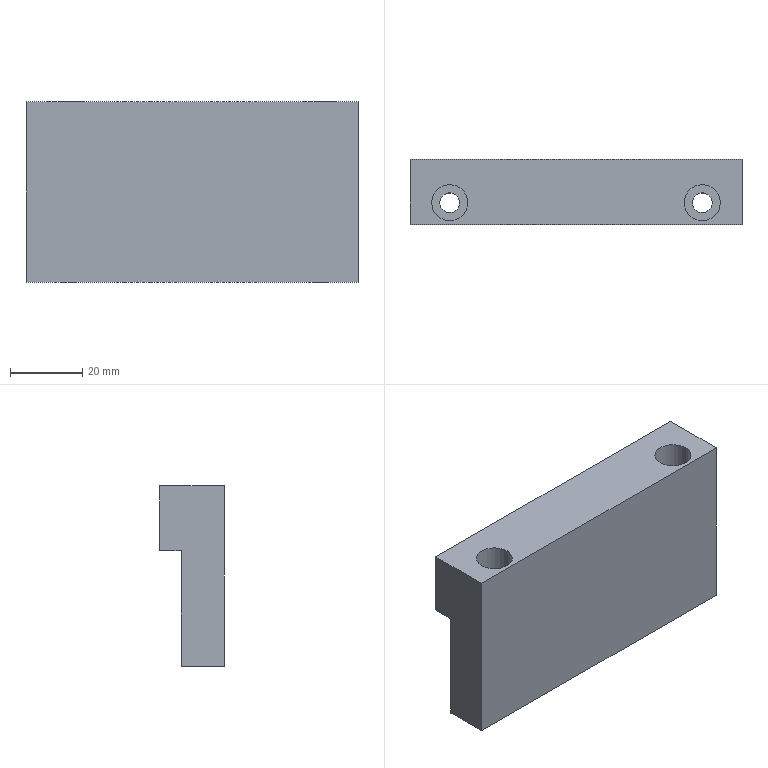Part | STEP file | 2081 Heat lower plate | 1 solid | 18 faces | box 92 x 18 x 50 mm | volume 61665 mm3 | plane 10 | cylinder 8 | commonest cylinder face diameters 5.5 x4 10 x4
STEP:
#1=CARTESIAN_POINT('',(0.,0.,0.));
#2=DIRECTION('',(0.,0.,1.));
#3=DIRECTION('',(1.,0.,0.));
#4=AXIS2_PLACEMENT_3D('',#1,#2,#3);
#5=CARTESIAN_POINT('',(-30.,-3.,8.));
#6=VERTEX_POINT('',#5);
#7=CARTESIAN_POINT('',(-30.,-3.,18.));
#8=VERTEX_POINT('',#7);
#9=CARTESIAN_POINT('',(-30.,-3.,18.));
#10=DIRECTION('',(0.,0.,1.));
#11=VECTOR('',#10,1.);
#12=LINE('',#9,#11);
#13=CARTESIAN_POINT('',(-35.,-3.,18.));
#14=DIRECTION('',(0.,0.,1.));
#15=DIRECTION('',(1.,0.,0.));
#16=AXIS2_PLACEMENT_3D('',#13,#14,#15);
#17=CYLINDRICAL_SURFACE('',#16,5.);
#18=CARTESIAN_POINT('',(6.283,0.));
#19=DIRECTION('',(0.,1.));
#20=VECTOR('',#19,1.);
#21=LINE('',#18,#20);
#22=(GEOMETRIC_REPRESENTATION_CONTEXT(2)PARAMETRIC_REPRESENTATION_CONTEXT()REPRESENTATION_CONTEXT('',''));
#23=DEFINITIONAL_REPRESENTATION('',(#21),#22);
#24=PCURVE('',#17,#23);
#25=CARTESIAN_POINT('',(-35.,-3.,18.));
#26=DIRECTION('',(0.,0.,1.));
#27=DIRECTION('',(1.,0.,0.));
#28=AXIS2_PLACEMENT_3D('',#25,#26,#27);
#29=CYLINDRICAL_SURFACE('',#28,5.);
#30=CARTESIAN_POINT('',(0.,0.));
#31=DIRECTION('',(0.,1.));
#32=VECTOR('',#31,1.);
#33=LINE('',#30,#32);
#34=(GEOMETRIC_REPRESENTATION_CONTEXT(2)PARAMETRIC_REPRESENTATION_CONTEXT()REPRESENTATION_CONTEXT('',''));
#35=DEFINITIONAL_REPRESENTATION('',(#33),#34);
#36=PCURVE('',#29,#35);
#37=SURFACE_CURVE('',#12,(#24,#36),.PCURVE_S1.);
#38=EDGE_CURVE('',#6,#8,#37,.T.);
#39=ORIENTED_EDGE('',*,*,#38,.T.);
#40=CARTESIAN_POINT('',(-40.,-3.,18.));
#41=VERTEX_POINT('',#40);
#42=CARTESIAN_POINT('',(-35.,-3.,18.));
#43=DIRECTION('',(0.,0.,1.));
#44=DIRECTION('',(1.,0.,0.));
#45=AXIS2_PLACEMENT_3D('',#42,#43,#44);
#46=CIRCLE('',#45,5.);
#47=CARTESIAN_POINT('',(0.,0.));
#48=DIRECTION('',(1.,0.));
#49=VECTOR('',#48,1.);
#50=LINE('',#47,#49);
#51=(GEOMETRIC_REPRESENTATION_CONTEXT(2)PARAMETRIC_REPRESENTATION_CONTEXT()REPRESENTATION_CONTEXT('',''));
#52=DEFINITIONAL_REPRESENTATION('',(#50),#51);
#53=PCURVE('',#17,#52);
#54=CARTESIAN_POINT('',(0.,0.,18.));
#55=DIRECTION('',(0.,0.,-1.));
#56=DIRECTION('',(-1.,0.,0.));
#57=AXIS2_PLACEMENT_3D('',#54,#55,#56);
#58=PLANE('',#57);
#59=CARTESIAN_POINT('',(30.,-3.));
#60=CARTESIAN_POINT('',(30.,5.66));
#61=CARTESIAN_POINT('',(37.5,1.33));
#62=CARTESIAN_POINT('',(45.,-3.));
#63=CARTESIAN_POINT('',(37.5,-7.33));
#64=CARTESIAN_POINT('',(30.,-11.66));
#65=CARTESIAN_POINT('',(30.,-3.));
#66=(BOUNDED_CURVE()B_SPLINE_CURVE(2,(#59,#60,#61,#62,#63,#64,#65),.UNSPECIFIED.,.T.,.F.)B_SPLINE_CURVE_WITH_KNOTS((1,2,2,2,2,1),(-2.094,0.,2.094,4.189,6.283,8.378),.UNSPECIFIED.)CURVE()GEOMETRIC_REPRESENTATION_ITEM()RATIONAL_B_SPLINE_CURVE((1.,0.5,1.,0.5,1.,0.5,1.))REPRESENTATION_ITEM(''));
#67=(GEOMETRIC_REPRESENTATION_CONTEXT(2)PARAMETRIC_REPRESENTATION_CONTEXT()REPRESENTATION_CONTEXT('',''));
#68=DEFINITIONAL_REPRESENTATION('',(#66),#67);
#69=PCURVE('',#58,#68);
#70=SURFACE_CURVE('',#46,(#53,#69),.PCURVE_S1.);
#71=EDGE_CURVE('',#41,#8,#70,.T.);
#72=ORIENTED_EDGE('',*,*,#71,.F.);
#73=CARTESIAN_POINT('',(-40.,-3.,8.));
#74=VERTEX_POINT('',#73);
#75=CARTESIAN_POINT('',(-40.,-3.,18.));
#76=DIRECTION('',(0.,0.,1.));
#77=VECTOR('',#76,1.);
#78=LINE('',#75,#77);
#79=CARTESIAN_POINT('',(3.142,0.));
#80=DIRECTION('',(0.,1.));
#81=VECTOR('',#80,1.);
#82=LINE('',#79,#81);
#83=(GEOMETRIC_REPRESENTATION_CONTEXT(2)PARAMETRIC_REPRESENTATION_CONTEXT()REPRESENTATION_CONTEXT('',''));
#84=DEFINITIONAL_REPRESENTATION('',(#82),#83);
#85=PCURVE('',#17,#84);
#86=CARTESIAN_POINT('',(3.142,0.));
#87=DIRECTION('',(0.,1.));
#88=VECTOR('',#87,1.);
#89=LINE('',#86,#88);
#90=(GEOMETRIC_REPRESENTATION_CONTEXT(2)PARAMETRIC_REPRESENTATION_CONTEXT()REPRESENTATION_CONTEXT('',''));
#91=DEFINITIONAL_REPRESENTATION('',(#89),#90);
#92=PCURVE('',#29,#91);
#93=SURFACE_CURVE('',#78,(#85,#92),.PCURVE_S1.);
#94=EDGE_CURVE('',#74,#41,#93,.T.);
#95=ORIENTED_EDGE('',*,*,#94,.F.);
#96=CARTESIAN_POINT('',(-35.,-3.,8.));
#97=DIRECTION('',(0.,0.,1.));
#98=DIRECTION('',(1.,0.,0.));
#99=AXIS2_PLACEMENT_3D('',#96,#97,#98);
#100=CIRCLE('',#99,5.);
#101=CARTESIAN_POINT('',(0.,-10.));
#102=DIRECTION('',(1.,0.));
#103=VECTOR('',#102,1.);
#104=LINE('',#101,#103);
#105=(GEOMETRIC_REPRESENTATION_CONTEXT(2)PARAMETRIC_REPRESENTATION_CONTEXT()REPRESENTATION_CONTEXT('',''));
#106=DEFINITIONAL_REPRESENTATION('',(#104),#105);
#107=PCURVE('',#17,#106);
#108=CARTESIAN_POINT('',(-32.25,-3.,8.));
#109=DIRECTION('',(0.,0.,-1.));
#110=DIRECTION('',(-1.,0.,0.));
#111=AXIS2_PLACEMENT_3D('',#108,#109,#110);
#112=PLANE('',#111);
#113=CARTESIAN_POINT('',(-2.25,0.));
#114=CARTESIAN_POINT('',(-2.25,8.66));
#115=CARTESIAN_POINT('',(5.25,4.33));
#116=CARTESIAN_POINT('',(12.75,0.));
#117=CARTESIAN_POINT('',(5.25,-4.33));
#118=CARTESIAN_POINT('',(-2.25,-8.66));
#119=CARTESIAN_POINT('',(-2.25,0.));
#120=(BOUNDED_CURVE()B_SPLINE_CURVE(2,(#113,#114,#115,#116,#117,#118,#119),.UNSPECIFIED.,.T.,.F.)B_SPLINE_CURVE_WITH_KNOTS((1,2,2,2,2,1),(-2.094,0.,2.094,4.189,6.283,8.378),.UNSPECIFIED.)CURVE()GEOMETRIC_REPRESENTATION_ITEM()RATIONAL_B_SPLINE_CURVE((1.,0.5,1.,0.5,1.,0.5,1.))REPRESENTATION_ITEM(''));
#121=(GEOMETRIC_REPRESENTATION_CONTEXT(2)PARAMETRIC_REPRESENTATION_CONTEXT()REPRESENTATION_CONTEXT('',''));
#122=DEFINITIONAL_REPRESENTATION('',(#120),#121);
#123=PCURVE('',#112,#122);
#124=SURFACE_CURVE('',#100,(#107,#123),.PCURVE_S1.);
#125=EDGE_CURVE('',#74,#6,#124,.T.);
#126=ORIENTED_EDGE('',*,*,#125,.T.);
#127=EDGE_LOOP('',(#39,#72,#95,#126));
#128=FACE_BOUND('',#127,.F.);
#129=ADVANCED_FACE('',(#128),#17,.F.);
#130=CARTESIAN_POINT('',(-32.25,-3.,-32.));
#131=VERTEX_POINT('',#130);
#132=CARTESIAN_POINT('',(-32.25,-3.,8.));
#133=VERTEX_POINT('',#132);
#134=CARTESIAN_POINT('',(-32.25,-3.,18.));
#135=DIRECTION('',(0.,0.,1.));
#136=VECTOR('',#135,1.);
#137=LINE('',#134,#136);
#138=CARTESIAN_POINT('',(-35.,-3.,18.));
#139=DIRECTION('',(0.,0.,1.));
#140=DIRECTION('',(1.,0.,0.));
#141=AXIS2_PLACEMENT_3D('',#138,#139,#140);
#142=CYLINDRICAL_SURFACE('',#141,2.75);
#143=CARTESIAN_POINT('',(6.283,0.));
#144=DIRECTION('',(0.,1.));
#145=VECTOR('',#144,1.);
#146=LINE('',#143,#145);
#147=(GEOMETRIC_REPRESENTATION_CONTEXT(2)PARAMETRIC_REPRESENTATION_CONTEXT()REPRESENTATION_CONTEXT('',''));
#148=DEFINITIONAL_REPRESENTATION('',(#146),#147);
#149=PCURVE('',#142,#148);
#150=CARTESIAN_POINT('',(-35.,-3.,18.));
#151=DIRECTION('',(0.,0.,1.));
#152=DIRECTION('',(1.,0.,0.));
#153=AXIS2_PLACEMENT_3D('',#150,#151,#152);
#154=CYLINDRICAL_SURFACE('',#153,2.75);
#155=CARTESIAN_POINT('',(0.,0.));
#156=DIRECTION('',(0.,1.));
#157=VECTOR('',#156,1.);
#158=LINE('',#155,#157);
#159=(GEOMETRIC_REPRESENTATION_CONTEXT(2)PARAMETRIC_REPRESENTATION_CONTEXT()REPRESENTATION_CONTEXT('',''));
#160=DEFINITIONAL_REPRESENTATION('',(#158),#159);
#161=PCURVE('',#154,#160);
#162=SURFACE_CURVE('',#137,(#149,#161),.PCURVE_S1.);
#163=EDGE_CURVE('',#131,#133,#162,.T.);
#164=ORIENTED_EDGE('',*,*,#163,.T.);
#165=CARTESIAN_POINT('',(-37.75,-3.,8.));
#166=VERTEX_POINT('',#165);
#167=CARTESIAN_POINT('',(-35.,-3.,8.));
#168=DIRECTION('',(0.,0.,1.));
#169=DIRECTION('',(1.,0.,0.));
#170=AXIS2_PLACEMENT_3D('',#167,#168,#169);
#171=CIRCLE('',#170,2.75);
#172=CARTESIAN_POINT('',(0.,-10.));
#173=DIRECTION('',(1.,0.));
#174=VECTOR('',#173,1.);
#175=LINE('',#172,#174);
#176=(GEOMETRIC_REPRESENTATION_CONTEXT(2)PARAMETRIC_REPRESENTATION_CONTEXT()REPRESENTATION_CONTEXT('',''));
#177=DEFINITIONAL_REPRESENTATION('',(#175),#176);
#178=PCURVE('',#142,#177);
#179=CARTESIAN_POINT('',(0.,0.));
#180=CARTESIAN_POINT('',(0.,4.763));
#181=CARTESIAN_POINT('',(4.125,2.382));
#182=CARTESIAN_POINT('',(8.25,0.));
#183=CARTESIAN_POINT('',(4.125,-2.382));
#184=CARTESIAN_POINT('',(0.,-4.763));
#185=CARTESIAN_POINT('',(0.,0.));
#186=(BOUNDED_CURVE()B_SPLINE_CURVE(2,(#179,#180,#181,#182,#183,#184,#185),.UNSPECIFIED.,.T.,.F.)B_SPLINE_CURVE_WITH_KNOTS((1,2,2,2,2,1),(-2.094,0.,2.094,4.189,6.283,8.378),.UNSPECIFIED.)CURVE()GEOMETRIC_REPRESENTATION_ITEM()RATIONAL_B_SPLINE_CURVE((1.,0.5,1.,0.5,1.,0.5,1.))REPRESENTATION_ITEM(''));
#187=(GEOMETRIC_REPRESENTATION_CONTEXT(2)PARAMETRIC_REPRESENTATION_CONTEXT()REPRESENTATION_CONTEXT('',''));
#188=DEFINITIONAL_REPRESENTATION('',(#186),#187);
#189=PCURVE('',#112,#188);
#190=SURFACE_CURVE('',#171,(#178,#189),.PCURVE_S1.);
#191=EDGE_CURVE('',#166,#133,#190,.T.);
#192=ORIENTED_EDGE('',*,*,#191,.F.);
#193=CARTESIAN_POINT('',(-37.75,-3.,-32.));
#194=VERTEX_POINT('',#193);
#195=CARTESIAN_POINT('',(-37.75,-3.,18.));
#196=DIRECTION('',(0.,0.,1.));
#197=VECTOR('',#196,1.);
#198=LINE('',#195,#197);
#199=CARTESIAN_POINT('',(3.142,0.));
#200=DIRECTION('',(0.,1.));
#201=VECTOR('',#200,1.);
#202=LINE('',#199,#201);
#203=(GEOMETRIC_REPRESENTATION_CONTEXT(2)PARAMETRIC_REPRESENTATION_CONTEXT()REPRESENTATION_CONTEXT('',''));
#204=DEFINITIONAL_REPRESENTATION('',(#202),#203);
#205=PCURVE('',#142,#204);
#206=CARTESIAN_POINT('',(3.142,0.));
#207=DIRECTION('',(0.,1.));
#208=VECTOR('',#207,1.);
#209=LINE('',#206,#208);
#210=(GEOMETRIC_REPRESENTATION_CONTEXT(2)PARAMETRIC_REPRESENTATION_CONTEXT()REPRESENTATION_CONTEXT('',''));
#211=DEFINITIONAL_REPRESENTATION('',(#209),#210);
#212=PCURVE('',#154,#211);
#213=SURFACE_CURVE('',#198,(#205,#212),.PCURVE_S1.);
#214=EDGE_CURVE('',#194,#166,#213,.T.);
#215=ORIENTED_EDGE('',*,*,#214,.F.);
#216=CARTESIAN_POINT('',(-35.,-3.,-32.));
#217=DIRECTION('',(0.,0.,1.));
#218=DIRECTION('',(1.,0.,0.));
#219=AXIS2_PLACEMENT_3D('',#216,#217,#218);
#220=CIRCLE('',#219,2.75);
#221=CARTESIAN_POINT('',(0.,-50.));
#222=DIRECTION('',(1.,0.));
#223=VECTOR('',#222,1.);
#224=LINE('',#221,#223);
#225=(GEOMETRIC_REPRESENTATION_CONTEXT(2)PARAMETRIC_REPRESENTATION_CONTEXT()REPRESENTATION_CONTEXT('',''));
#226=DEFINITIONAL_REPRESENTATION('',(#224),#225);
#227=PCURVE('',#142,#226);
#228=CARTESIAN_POINT('',(0.,0.,-32.));
#229=DIRECTION('',(0.,0.,1.));
#230=DIRECTION('',(1.,0.,0.));
#231=AXIS2_PLACEMENT_3D('',#228,#229,#230);
#232=PLANE('',#231);
#233=CARTESIAN_POINT('',(-35.,-3.));
#234=DIRECTION('',(1.,0.));
#235=AXIS2_PLACEMENT_2D('',#233,#234);
#236=CIRCLE('',#235,2.75);
#237=(GEOMETRIC_REPRESENTATION_CONTEXT(2)PARAMETRIC_REPRESENTATION_CONTEXT()REPRESENTATION_CONTEXT('',''));
#238=DEFINITIONAL_REPRESENTATION('',(#236),#237);
#239=PCURVE('',#232,#238);
#240=SURFACE_CURVE('',#220,(#227,#239),.PCURVE_S1.);
#241=EDGE_CURVE('',#194,#131,#240,.T.);
#242=ORIENTED_EDGE('',*,*,#241,.T.);
#243=EDGE_LOOP('',(#164,#192,#215,#242));
#244=FACE_BOUND('',#243,.F.);
#245=ADVANCED_FACE('',(#244),#142,.F.);
#246=CARTESIAN_POINT('',(40.,-3.,8.));
#247=VERTEX_POINT('',#246);
#248=CARTESIAN_POINT('',(40.,-3.,18.));
#249=VERTEX_POINT('',#248);
#250=CARTESIAN_POINT('',(40.,-3.,18.));
#251=DIRECTION('',(0.,0.,1.));
#252=VECTOR('',#251,1.);
#253=LINE('',#250,#252);
#254=CARTESIAN_POINT('',(35.,-3.,18.));
#255=DIRECTION('',(0.,0.,1.));
#256=DIRECTION('',(1.,0.,0.));
#257=AXIS2_PLACEMENT_3D('',#254,#255,#256);
#258=CYLINDRICAL_SURFACE('',#257,5.);
#259=CARTESIAN_POINT('',(6.283,0.));
#260=DIRECTION('',(0.,1.));
#261=VECTOR('',#260,1.);
#262=LINE('',#259,#261);
#263=(GEOMETRIC_REPRESENTATION_CONTEXT(2)PARAMETRIC_REPRESENTATION_CONTEXT()REPRESENTATION_CONTEXT('',''));
#264=DEFINITIONAL_REPRESENTATION('',(#262),#263);
#265=PCURVE('',#258,#264);
#266=CARTESIAN_POINT('',(35.,-3.,18.));
#267=DIRECTION('',(0.,0.,1.));
#268=DIRECTION('',(1.,0.,0.));
#269=AXIS2_PLACEMENT_3D('',#266,#267,#268);
#270=CYLINDRICAL_SURFACE('',#269,5.);
#271=CARTESIAN_POINT('',(0.,0.));
#272=DIRECTION('',(0.,1.));
#273=VECTOR('',#272,1.);
#274=LINE('',#271,#273);
#275=(GEOMETRIC_REPRESENTATION_CONTEXT(2)PARAMETRIC_REPRESENTATION_CONTEXT()REPRESENTATION_CONTEXT('',''));
#276=DEFINITIONAL_REPRESENTATION('',(#274),#275);
#277=PCURVE('',#270,#276);
#278=SURFACE_CURVE('',#253,(#265,#277),.PCURVE_S1.);
#279=EDGE_CURVE('',#247,#249,#278,.T.);
#280=ORIENTED_EDGE('',*,*,#279,.T.);
#281=CARTESIAN_POINT('',(30.,-3.,18.));
#282=VERTEX_POINT('',#281);
#283=CARTESIAN_POINT('',(35.,-3.,18.));
#284=DIRECTION('',(0.,0.,1.));
#285=DIRECTION('',(1.,0.,0.));
#286=AXIS2_PLACEMENT_3D('',#283,#284,#285);
#287=CIRCLE('',#286,5.);
#288=CARTESIAN_POINT('',(0.,0.));
#289=DIRECTION('',(1.,0.));
#290=VECTOR('',#289,1.);
#291=LINE('',#288,#290);
#292=(GEOMETRIC_REPRESENTATION_CONTEXT(2)PARAMETRIC_REPRESENTATION_CONTEXT()REPRESENTATION_CONTEXT('',''));
#293=DEFINITIONAL_REPRESENTATION('',(#291),#292);
#294=PCURVE('',#258,#293);
#295=CARTESIAN_POINT('',(-40.,-3.));
#296=CARTESIAN_POINT('',(-40.,5.66));
#297=CARTESIAN_POINT('',(-32.5,1.33));
#298=CARTESIAN_POINT('',(-25.,-3.));
#299=CARTESIAN_POINT('',(-32.5,-7.33));
#300=CARTESIAN_POINT('',(-40.,-11.66));
#301=CARTESIAN_POINT('',(-40.,-3.));
#302=(BOUNDED_CURVE()B_SPLINE_CURVE(2,(#295,#296,#297,#298,#299,#300,#301),.UNSPECIFIED.,.T.,.F.)B_SPLINE_CURVE_WITH_KNOTS((1,2,2,2,2,1),(-2.094,0.,2.094,4.189,6.283,8.378),.UNSPECIFIED.)CURVE()GEOMETRIC_REPRESENTATION_ITEM()RATIONAL_B_SPLINE_CURVE((1.,0.5,1.,0.5,1.,0.5,1.))REPRESENTATION_ITEM(''));
#303=(GEOMETRIC_REPRESENTATION_CONTEXT(2)PARAMETRIC_REPRESENTATION_CONTEXT()REPRESENTATION_CONTEXT('',''));
#304=DEFINITIONAL_REPRESENTATION('',(#302),#303);
#305=PCURVE('',#58,#304);
#306=SURFACE_CURVE('',#287,(#294,#305),.PCURVE_S1.);
#307=EDGE_CURVE('',#282,#249,#306,.T.);
#308=ORIENTED_EDGE('',*,*,#307,.F.);
#309=CARTESIAN_POINT('',(30.,-3.,8.));
#310=VERTEX_POINT('',#309);
#311=CARTESIAN_POINT('',(30.,-3.,18.));
#312=DIRECTION('',(0.,0.,1.));
#313=VECTOR('',#312,1.);
#314=LINE('',#311,#313);
#315=CARTESIAN_POINT('',(3.142,0.));
#316=DIRECTION('',(0.,1.));
#317=VECTOR('',#316,1.);
#318=LINE('',#315,#317);
#319=(GEOMETRIC_REPRESENTATION_CONTEXT(2)PARAMETRIC_REPRESENTATION_CONTEXT()REPRESENTATION_CONTEXT('',''));
#320=DEFINITIONAL_REPRESENTATION('',(#318),#319);
#321=PCURVE('',#258,#320);
#322=CARTESIAN_POINT('',(3.142,0.));
#323=DIRECTION('',(0.,1.));
#324=VECTOR('',#323,1.);
#325=LINE('',#322,#324);
#326=(GEOMETRIC_REPRESENTATION_CONTEXT(2)PARAMETRIC_REPRESENTATION_CONTEXT()REPRESENTATION_CONTEXT('',''));
#327=DEFINITIONAL_REPRESENTATION('',(#325),#326);
#328=PCURVE('',#270,#327);
#329=SURFACE_CURVE('',#314,(#321,#328),.PCURVE_S1.);
#330=EDGE_CURVE('',#310,#282,#329,.T.);
#331=ORIENTED_EDGE('',*,*,#330,.F.);
#332=CARTESIAN_POINT('',(35.,-3.,8.));
#333=DIRECTION('',(0.,0.,1.));
#334=DIRECTION('',(1.,0.,0.));
#335=AXIS2_PLACEMENT_3D('',#332,#333,#334);
#336=CIRCLE('',#335,5.);
#337=CARTESIAN_POINT('',(0.,-10.));
#338=DIRECTION('',(1.,0.));
#339=VECTOR('',#338,1.);
#340=LINE('',#337,#339);
#341=(GEOMETRIC_REPRESENTATION_CONTEXT(2)PARAMETRIC_REPRESENTATION_CONTEXT()REPRESENTATION_CONTEXT('',''));
#342=DEFINITIONAL_REPRESENTATION('',(#340),#341);
#343=PCURVE('',#258,#342);
#344=CARTESIAN_POINT('',(37.75,-3.,8.));
#345=DIRECTION('',(0.,0.,-1.));
#346=DIRECTION('',(-1.,0.,0.));
#347=AXIS2_PLACEMENT_3D('',#344,#345,#346);
#348=PLANE('',#347);
#349=CARTESIAN_POINT('',(-2.25,0.));
#350=CARTESIAN_POINT('',(-2.25,8.66));
#351=CARTESIAN_POINT('',(5.25,4.33));
#352=CARTESIAN_POINT('',(12.75,0.));
#353=CARTESIAN_POINT('',(5.25,-4.33));
#354=CARTESIAN_POINT('',(-2.25,-8.66));
#355=CARTESIAN_POINT('',(-2.25,0.));
#356=(BOUNDED_CURVE()B_SPLINE_CURVE(2,(#349,#350,#351,#352,#353,#354,#355),.UNSPECIFIED.,.T.,.F.)B_SPLINE_CURVE_WITH_KNOTS((1,2,2,2,2,1),(-2.094,0.,2.094,4.189,6.283,8.378),.UNSPECIFIED.)CURVE()GEOMETRIC_REPRESENTATION_ITEM()RATIONAL_B_SPLINE_CURVE((1.,0.5,1.,0.5,1.,0.5,1.))REPRESENTATION_ITEM(''));
#357=(GEOMETRIC_REPRESENTATION_CONTEXT(2)PARAMETRIC_REPRESENTATION_CONTEXT()REPRESENTATION_CONTEXT('',''));
#358=DEFINITIONAL_REPRESENTATION('',(#356),#357);
#359=PCURVE('',#348,#358);
#360=SURFACE_CURVE('',#336,(#343,#359),.PCURVE_S1.);
#361=EDGE_CURVE('',#310,#247,#360,.T.);
#362=ORIENTED_EDGE('',*,*,#361,.T.);
#363=EDGE_LOOP('',(#280,#308,#331,#362));
#364=FACE_BOUND('',#363,.F.);
#365=ADVANCED_FACE('',(#364),#258,.F.);
#366=CARTESIAN_POINT('',(37.75,-3.,-32.));
#367=VERTEX_POINT('',#366);
#368=CARTESIAN_POINT('',(37.75,-3.,8.));
#369=VERTEX_POINT('',#368);
#370=CARTESIAN_POINT('',(37.75,-3.,18.));
#371=DIRECTION('',(0.,0.,1.));
#372=VECTOR('',#371,1.);
#373=LINE('',#370,#372);
#374=CARTESIAN_POINT('',(35.,-3.,18.));
#375=DIRECTION('',(0.,0.,1.));
#376=DIRECTION('',(1.,0.,0.));
#377=AXIS2_PLACEMENT_3D('',#374,#375,#376);
#378=CYLINDRICAL_SURFACE('',#377,2.75);
#379=CARTESIAN_POINT('',(6.283,0.));
#380=DIRECTION('',(0.,1.));
#381=VECTOR('',#380,1.);
#382=LINE('',#379,#381);
#383=(GEOMETRIC_REPRESENTATION_CONTEXT(2)PARAMETRIC_REPRESENTATION_CONTEXT()REPRESENTATION_CONTEXT('',''));
#384=DEFINITIONAL_REPRESENTATION('',(#382),#383);
#385=PCURVE('',#378,#384);
#386=CARTESIAN_POINT('',(35.,-3.,18.));
#387=DIRECTION('',(0.,0.,1.));
#388=DIRECTION('',(1.,0.,0.));
#389=AXIS2_PLACEMENT_3D('',#386,#387,#388);
#390=CYLINDRICAL_SURFACE('',#389,2.75);
#391=CARTESIAN_POINT('',(0.,0.));
#392=DIRECTION('',(0.,1.));
#393=VECTOR('',#392,1.);
#394=LINE('',#391,#393);
#395=(GEOMETRIC_REPRESENTATION_CONTEXT(2)PARAMETRIC_REPRESENTATION_CONTEXT()REPRESENTATION_CONTEXT('',''));
#396=DEFINITIONAL_REPRESENTATION('',(#394),#395);
#397=PCURVE('',#390,#396);
#398=SURFACE_CURVE('',#373,(#385,#397),.PCURVE_S1.);
#399=EDGE_CURVE('',#367,#369,#398,.T.);
#400=ORIENTED_EDGE('',*,*,#399,.T.);
#401=CARTESIAN_POINT('',(32.25,-3.,8.));
#402=VERTEX_POINT('',#401);
#403=CARTESIAN_POINT('',(35.,-3.,8.));
#404=DIRECTION('',(0.,0.,1.));
#405=DIRECTION('',(1.,0.,0.));
#406=AXIS2_PLACEMENT_3D('',#403,#404,#405);
#407=CIRCLE('',#406,2.75);
#408=CARTESIAN_POINT('',(0.,-10.));
#409=DIRECTION('',(1.,0.));
#410=VECTOR('',#409,1.);
#411=LINE('',#408,#410);
#412=(GEOMETRIC_REPRESENTATION_CONTEXT(2)PARAMETRIC_REPRESENTATION_CONTEXT()REPRESENTATION_CONTEXT('',''));
#413=DEFINITIONAL_REPRESENTATION('',(#411),#412);
#414=PCURVE('',#378,#413);
#415=CARTESIAN_POINT('',(0.,0.));
#416=CARTESIAN_POINT('',(0.,4.763));
#417=CARTESIAN_POINT('',(4.125,2.382));
#418=CARTESIAN_POINT('',(8.25,0.));
#419=CARTESIAN_POINT('',(4.125,-2.382));
#420=CARTESIAN_POINT('',(0.,-4.763));
#421=CARTESIAN_POINT('',(0.,0.));
#422=(BOUNDED_CURVE()B_SPLINE_CURVE(2,(#415,#416,#417,#418,#419,#420,#421),.UNSPECIFIED.,.T.,.F.)B_SPLINE_CURVE_WITH_KNOTS((1,2,2,2,2,1),(-2.094,0.,2.094,4.189,6.283,8.378),.UNSPECIFIED.)CURVE()GEOMETRIC_REPRESENTATION_ITEM()RATIONAL_B_SPLINE_CURVE((1.,0.5,1.,0.5,1.,0.5,1.))REPRESENTATION_ITEM(''));
#423=(GEOMETRIC_REPRESENTATION_CONTEXT(2)PARAMETRIC_REPRESENTATION_CONTEXT()REPRESENTATION_CONTEXT('',''));
#424=DEFINITIONAL_REPRESENTATION('',(#422),#423);
#425=PCURVE('',#348,#424);
#426=SURFACE_CURVE('',#407,(#414,#425),.PCURVE_S1.);
#427=EDGE_CURVE('',#402,#369,#426,.T.);
#428=ORIENTED_EDGE('',*,*,#427,.F.);
#429=CARTESIAN_POINT('',(32.25,-3.,-32.));
#430=VERTEX_POINT('',#429);
#431=CARTESIAN_POINT('',(32.25,-3.,18.));
#432=DIRECTION('',(0.,0.,1.));
#433=VECTOR('',#432,1.);
#434=LINE('',#431,#433);
#435=CARTESIAN_POINT('',(3.142,0.));
#436=DIRECTION('',(0.,1.));
#437=VECTOR('',#436,1.);
#438=LINE('',#435,#437);
#439=(GEOMETRIC_REPRESENTATION_CONTEXT(2)PARAMETRIC_REPRESENTATION_CONTEXT()REPRESENTATION_CONTEXT('',''));
#440=DEFINITIONAL_REPRESENTATION('',(#438),#439);
#441=PCURVE('',#378,#440);
#442=CARTESIAN_POINT('',(3.142,0.));
#443=DIRECTION('',(0.,1.));
#444=VECTOR('',#443,1.);
#445=LINE('',#442,#444);
#446=(GEOMETRIC_REPRESENTATION_CONTEXT(2)PARAMETRIC_REPRESENTATION_CONTEXT()REPRESENTATION_CONTEXT('',''));
#447=DEFINITIONAL_REPRESENTATION('',(#445),#446);
#448=PCURVE('',#390,#447);
#449=SURFACE_CURVE('',#434,(#441,#448),.PCURVE_S1.);
#450=EDGE_CURVE('',#430,#402,#449,.T.);
#451=ORIENTED_EDGE('',*,*,#450,.F.);
#452=CARTESIAN_POINT('',(35.,-3.,-32.));
#453=DIRECTION('',(0.,0.,1.));
#454=DIRECTION('',(1.,0.,0.));
#455=AXIS2_PLACEMENT_3D('',#452,#453,#454);
#456=CIRCLE('',#455,2.75);
#457=CARTESIAN_POINT('',(0.,-50.));
#458=DIRECTION('',(1.,0.));
#459=VECTOR('',#458,1.);
#460=LINE('',#457,#459);
#461=(GEOMETRIC_REPRESENTATION_CONTEXT(2)PARAMETRIC_REPRESENTATION_CONTEXT()REPRESENTATION_CONTEXT('',''));
#462=DEFINITIONAL_REPRESENTATION('',(#460),#461);
#463=PCURVE('',#378,#462);
#464=CARTESIAN_POINT('',(35.,-3.));
#465=DIRECTION('',(1.,0.));
#466=AXIS2_PLACEMENT_2D('',#464,#465);
#467=CIRCLE('',#466,2.75);
#468=(GEOMETRIC_REPRESENTATION_CONTEXT(2)PARAMETRIC_REPRESENTATION_CONTEXT()REPRESENTATION_CONTEXT('',''));
#469=DEFINITIONAL_REPRESENTATION('',(#467),#468);
#470=PCURVE('',#232,#469);
#471=SURFACE_CURVE('',#456,(#463,#470),.PCURVE_S1.);
#472=EDGE_CURVE('',#430,#367,#471,.T.);
#473=ORIENTED_EDGE('',*,*,#472,.T.);
#474=EDGE_LOOP('',(#400,#428,#451,#473));
#475=FACE_BOUND('',#474,.F.);
#476=ADVANCED_FACE('',(#475),#378,.F.);
#477=CARTESIAN_POINT('',(46.,-9.,18.));
#478=VERTEX_POINT('',#477);
#479=CARTESIAN_POINT('',(46.,-9.,-32.));
#480=VERTEX_POINT('',#479);
#481=CARTESIAN_POINT('',(46.,-9.,18.));
#482=DIRECTION('',(0.,0.,-1.));
#483=VECTOR('',#482,1.);
#484=LINE('',#481,#483);
#485=CARTESIAN_POINT('',(46.,-9.,18.));
#486=DIRECTION('',(-1.,0.,0.));
#487=DIRECTION('',(0.,0.,1.));
#488=AXIS2_PLACEMENT_3D('',#485,#486,#487);
#489=PLANE('',#488);
#490=CARTESIAN_POINT('',(0.,0.));
#491=DIRECTION('',(-1.,0.));
#492=VECTOR('',#491,1.);
#493=LINE('',#490,#492);
#494=(GEOMETRIC_REPRESENTATION_CONTEXT(2)PARAMETRIC_REPRESENTATION_CONTEXT()REPRESENTATION_CONTEXT('',''));
#495=DEFINITIONAL_REPRESENTATION('',(#493),#494);
#496=PCURVE('',#489,#495);
#497=CARTESIAN_POINT('',(-46.,-9.,18.));
#498=DIRECTION('',(0.,1.,0.));
#499=DIRECTION('',(0.,0.,1.));
#500=AXIS2_PLACEMENT_3D('',#497,#498,#499);
#501=PLANE('',#500);
#502=CARTESIAN_POINT('',(0.,92.));
#503=DIRECTION('',(-1.,0.));
#504=VECTOR('',#503,1.);
#505=LINE('',#502,#504);
#506=(GEOMETRIC_REPRESENTATION_CONTEXT(2)PARAMETRIC_REPRESENTATION_CONTEXT()REPRESENTATION_CONTEXT('',''));
#507=DEFINITIONAL_REPRESENTATION('',(#505),#506);
#508=PCURVE('',#501,#507);
#509=SURFACE_CURVE('',#484,(#496,#508),.PCURVE_S1.);
#510=EDGE_CURVE('',#478,#480,#509,.T.);
#511=ORIENTED_EDGE('',*,*,#510,.T.);
#512=CARTESIAN_POINT('',(46.,3.,-32.));
#513=VERTEX_POINT('',#512);
#514=CARTESIAN_POINT('',(46.,-9.,-32.));
#515=DIRECTION('',(0.,-1.,0.));
#516=VECTOR('',#515,1.);
#517=LINE('',#514,#516);
#518=CARTESIAN_POINT('',(-50.,0.));
#519=DIRECTION('',(0.,-1.));
#520=VECTOR('',#519,1.);
#521=LINE('',#518,#520);
#522=(GEOMETRIC_REPRESENTATION_CONTEXT(2)PARAMETRIC_REPRESENTATION_CONTEXT()REPRESENTATION_CONTEXT('',''));
#523=DEFINITIONAL_REPRESENTATION('',(#521),#522);
#524=PCURVE('',#489,#523);
#525=CARTESIAN_POINT('',(46.,-9.));
#526=DIRECTION('',(0.,-1.));
#527=VECTOR('',#526,1.);
#528=LINE('',#525,#527);
#529=(GEOMETRIC_REPRESENTATION_CONTEXT(2)PARAMETRIC_REPRESENTATION_CONTEXT()REPRESENTATION_CONTEXT('',''));
#530=DEFINITIONAL_REPRESENTATION('',(#528),#529);
#531=PCURVE('',#232,#530);
#532=SURFACE_CURVE('',#517,(#524,#531),.PCURVE_S1.);
#533=EDGE_CURVE('',#513,#480,#532,.T.);
#534=ORIENTED_EDGE('',*,*,#533,.F.);
#535=CARTESIAN_POINT('',(46.,3.,0.));
#536=VERTEX_POINT('',#535);
#537=CARTESIAN_POINT('',(46.,3.,-32.));
#538=DIRECTION('',(0.,0.,1.));
#539=VECTOR('',#538,1.);
#540=LINE('',#537,#539);
#541=CARTESIAN_POINT('',(-50.,12.));
#542=DIRECTION('',(1.,0.));
#543=VECTOR('',#542,1.);
#544=LINE('',#541,#543);
#545=(GEOMETRIC_REPRESENTATION_CONTEXT(2)PARAMETRIC_REPRESENTATION_CONTEXT()REPRESENTATION_CONTEXT('',''));
#546=DEFINITIONAL_REPRESENTATION('',(#544),#545);
#547=PCURVE('',#489,#546);
#548=CARTESIAN_POINT('',(46.,3.,-32.));
#549=DIRECTION('',(0.,-1.,0.));
#550=DIRECTION('',(0.,0.,-1.));
#551=AXIS2_PLACEMENT_3D('',#548,#549,#550);
#552=PLANE('',#551);
#553=CARTESIAN_POINT('',(0.,0.));
#554=DIRECTION('',(-1.,0.));
#555=VECTOR('',#554,1.);
#556=LINE('',#553,#555);
#557=(GEOMETRIC_REPRESENTATION_CONTEXT(2)PARAMETRIC_REPRESENTATION_CONTEXT()REPRESENTATION_CONTEXT('',''));
#558=DEFINITIONAL_REPRESENTATION('',(#556),#557);
#559=PCURVE('',#552,#558);
#560=SURFACE_CURVE('',#540,(#547,#559),.PCURVE_S1.);
#561=EDGE_CURVE('',#513,#536,#560,.T.);
#562=ORIENTED_EDGE('',*,*,#561,.T.);
#563=CARTESIAN_POINT('',(46.,9.,0.));
#564=VERTEX_POINT('',#563);
#565=CARTESIAN_POINT('',(46.,-9.,0.));
#566=DIRECTION('',(0.,1.,0.));
#567=VECTOR('',#566,1.);
#568=LINE('',#565,#567);
#569=CARTESIAN_POINT('',(-18.,0.));
#570=DIRECTION('',(0.,1.));
#571=VECTOR('',#570,1.);
#572=LINE('',#569,#571);
#573=(GEOMETRIC_REPRESENTATION_CONTEXT(2)PARAMETRIC_REPRESENTATION_CONTEXT()REPRESENTATION_CONTEXT('',''));
#574=DEFINITIONAL_REPRESENTATION('',(#572),#573);
#575=PCURVE('',#489,#574);
#576=CARTESIAN_POINT('',(0.,0.,0.));
#577=DIRECTION('',(0.,0.,-1.));
#578=DIRECTION('',(-1.,0.,0.));
#579=AXIS2_PLACEMENT_3D('',#576,#577,#578);
#580=PLANE('',#579);
#581=CARTESIAN_POINT('',(-46.,-9.));
#582=DIRECTION('',(0.,1.));
#583=VECTOR('',#582,1.);
#584=LINE('',#581,#583);
#585=(GEOMETRIC_REPRESENTATION_CONTEXT(2)PARAMETRIC_REPRESENTATION_CONTEXT()REPRESENTATION_CONTEXT('',''));
#586=DEFINITIONAL_REPRESENTATION('',(#584),#585);
#587=PCURVE('',#580,#586);
#588=SURFACE_CURVE('',#568,(#575,#587),.PCURVE_S1.);
#589=EDGE_CURVE('',#536,#564,#588,.T.);
#590=ORIENTED_EDGE('',*,*,#589,.T.);
#591=CARTESIAN_POINT('',(46.,9.,18.));
#592=VERTEX_POINT('',#591);
#593=CARTESIAN_POINT('',(46.,9.,18.));
#594=DIRECTION('',(0.,0.,-1.));
#595=VECTOR('',#594,1.);
#596=LINE('',#593,#595);
#597=CARTESIAN_POINT('',(0.,18.));
#598=DIRECTION('',(-1.,0.));
#599=VECTOR('',#598,1.);
#600=LINE('',#597,#599);
#601=(GEOMETRIC_REPRESENTATION_CONTEXT(2)PARAMETRIC_REPRESENTATION_CONTEXT()REPRESENTATION_CONTEXT('',''));
#602=DEFINITIONAL_REPRESENTATION('',(#600),#601);
#603=PCURVE('',#489,#602);
#604=CARTESIAN_POINT('',(-46.,9.,18.));
#605=DIRECTION('',(0.,-1.,0.));
#606=DIRECTION('',(0.,0.,-1.));
#607=AXIS2_PLACEMENT_3D('',#604,#605,#606);
#608=PLANE('',#607);
#609=CARTESIAN_POINT('',(0.,92.));
#610=DIRECTION('',(1.,0.));
#611=VECTOR('',#610,1.);
#612=LINE('',#609,#611);
#613=(GEOMETRIC_REPRESENTATION_CONTEXT(2)PARAMETRIC_REPRESENTATION_CONTEXT()REPRESENTATION_CONTEXT('',''));
#614=DEFINITIONAL_REPRESENTATION('',(#612),#613);
#615=PCURVE('',#608,#614);
#616=SURFACE_CURVE('',#596,(#603,#615),.PCURVE_S1.);
#617=EDGE_CURVE('',#592,#564,#616,.T.);
#618=ORIENTED_EDGE('',*,*,#617,.F.);
#619=CARTESIAN_POINT('',(46.,-9.,18.));
#620=DIRECTION('',(0.,1.,0.));
#621=VECTOR('',#620,1.);
#622=LINE('',#619,#621);
#623=CARTESIAN_POINT('',(0.,0.));
#624=DIRECTION('',(0.,1.));
#625=VECTOR('',#624,1.);
#626=LINE('',#623,#625);
#627=(GEOMETRIC_REPRESENTATION_CONTEXT(2)PARAMETRIC_REPRESENTATION_CONTEXT()REPRESENTATION_CONTEXT('',''));
#628=DEFINITIONAL_REPRESENTATION('',(#626),#627);
#629=PCURVE('',#489,#628);
#630=CARTESIAN_POINT('',(-46.,-9.));
#631=DIRECTION('',(0.,1.));
#632=VECTOR('',#631,1.);
#633=LINE('',#630,#632);
#634=(GEOMETRIC_REPRESENTATION_CONTEXT(2)PARAMETRIC_REPRESENTATION_CONTEXT()REPRESENTATION_CONTEXT('',''));
#635=DEFINITIONAL_REPRESENTATION('',(#633),#634);
#636=PCURVE('',#58,#635);
#637=SURFACE_CURVE('',#622,(#629,#636),.PCURVE_S1.);
#638=EDGE_CURVE('',#478,#592,#637,.T.);
#639=ORIENTED_EDGE('',*,*,#638,.F.);
#640=EDGE_LOOP('',(#511,#534,#562,#590,#618,#639));
#641=FACE_BOUND('',#640,.T.);
#642=ADVANCED_FACE('',(#641),#489,.F.);
#643=CARTESIAN_POINT('',(-46.,9.,0.));
#644=VERTEX_POINT('',#643);
#645=CARTESIAN_POINT('',(-46.,9.,0.));
#646=DIRECTION('',(-1.,0.,0.));
#647=VECTOR('',#646,1.);
#648=LINE('',#645,#647);
#649=CARTESIAN_POINT('',(18.,0.));
#650=DIRECTION('',(0.,-1.));
#651=VECTOR('',#650,1.);
#652=LINE('',#649,#651);
#653=(GEOMETRIC_REPRESENTATION_CONTEXT(2)PARAMETRIC_REPRESENTATION_CONTEXT()REPRESENTATION_CONTEXT('',''));
#654=DEFINITIONAL_REPRESENTATION('',(#652),#653);
#655=PCURVE('',#608,#654);
#656=CARTESIAN_POINT('',(46.,9.));
#657=DIRECTION('',(1.,0.));
#658=VECTOR('',#657,1.);
#659=LINE('',#656,#658);
#660=(GEOMETRIC_REPRESENTATION_CONTEXT(2)PARAMETRIC_REPRESENTATION_CONTEXT()REPRESENTATION_CONTEXT('',''));
#661=DEFINITIONAL_REPRESENTATION('',(#659),#660);
#662=PCURVE('',#580,#661);
#663=SURFACE_CURVE('',#648,(#655,#662),.PCURVE_S1.);
#664=EDGE_CURVE('',#564,#644,#663,.T.);
#665=ORIENTED_EDGE('',*,*,#664,.T.);
#666=CARTESIAN_POINT('',(-46.,9.,18.));
#667=VERTEX_POINT('',#666);
#668=CARTESIAN_POINT('',(-46.,9.,18.));
#669=DIRECTION('',(0.,0.,-1.));
#670=VECTOR('',#669,1.);
#671=LINE('',#668,#670);
#672=CARTESIAN_POINT('',(0.,0.));
#673=DIRECTION('',(1.,0.));
#674=VECTOR('',#673,1.);
#675=LINE('',#672,#674);
#676=(GEOMETRIC_REPRESENTATION_CONTEXT(2)PARAMETRIC_REPRESENTATION_CONTEXT()REPRESENTATION_CONTEXT('',''));
#677=DEFINITIONAL_REPRESENTATION('',(#675),#676);
#678=PCURVE('',#608,#677);
#679=CARTESIAN_POINT('',(-46.,-9.,18.));
#680=DIRECTION('',(1.,0.,0.));
#681=DIRECTION('',(0.,0.,-1.));
#682=AXIS2_PLACEMENT_3D('',#679,#680,#681);
#683=PLANE('',#682);
#684=CARTESIAN_POINT('',(0.,18.));
#685=DIRECTION('',(1.,0.));
#686=VECTOR('',#685,1.);
#687=LINE('',#684,#686);
#688=(GEOMETRIC_REPRESENTATION_CONTEXT(2)PARAMETRIC_REPRESENTATION_CONTEXT()REPRESENTATION_CONTEXT('',''));
#689=DEFINITIONAL_REPRESENTATION('',(#687),#688);
#690=PCURVE('',#683,#689);
#691=SURFACE_CURVE('',#671,(#678,#690),.PCURVE_S1.);
#692=EDGE_CURVE('',#667,#644,#691,.T.);
#693=ORIENTED_EDGE('',*,*,#692,.F.);
#694=CARTESIAN_POINT('',(-46.,9.,18.));
#695=DIRECTION('',(-1.,0.,0.));
#696=VECTOR('',#695,1.);
#697=LINE('',#694,#696);
#698=CARTESIAN_POINT('',(0.,0.));
#699=DIRECTION('',(0.,-1.));
#700=VECTOR('',#699,1.);
#701=LINE('',#698,#700);
#702=(GEOMETRIC_REPRESENTATION_CONTEXT(2)PARAMETRIC_REPRESENTATION_CONTEXT()REPRESENTATION_CONTEXT('',''));
#703=DEFINITIONAL_REPRESENTATION('',(#701),#702);
#704=PCURVE('',#608,#703);
#705=CARTESIAN_POINT('',(46.,9.));
#706=DIRECTION('',(1.,0.));
#707=VECTOR('',#706,1.);
#708=LINE('',#705,#707);
#709=(GEOMETRIC_REPRESENTATION_CONTEXT(2)PARAMETRIC_REPRESENTATION_CONTEXT()REPRESENTATION_CONTEXT('',''));
#710=DEFINITIONAL_REPRESENTATION('',(#708),#709);
#711=PCURVE('',#58,#710);
#712=SURFACE_CURVE('',#697,(#704,#711),.PCURVE_S1.);
#713=EDGE_CURVE('',#592,#667,#712,.T.);
#714=ORIENTED_EDGE('',*,*,#713,.F.);
#715=ORIENTED_EDGE('',*,*,#617,.T.);
#716=EDGE_LOOP('',(#665,#693,#714,#715));
#717=FACE_BOUND('',#716,.T.);
#718=ADVANCED_FACE('',(#717),#608,.F.);
#719=CARTESIAN_POINT('',(-46.,3.,0.));
#720=VERTEX_POINT('',#719);
#721=CARTESIAN_POINT('',(-46.,-9.,0.));
#722=DIRECTION('',(0.,-1.,0.));
#723=VECTOR('',#722,1.);
#724=LINE('',#721,#723);
#725=CARTESIAN_POINT('',(18.,0.));
#726=DIRECTION('',(0.,-1.));
#727=VECTOR('',#726,1.);
#728=LINE('',#725,#727);
#729=(GEOMETRIC_REPRESENTATION_CONTEXT(2)PARAMETRIC_REPRESENTATION_CONTEXT()REPRESENTATION_CONTEXT('',''));
#730=DEFINITIONAL_REPRESENTATION('',(#728),#729);
#731=PCURVE('',#683,#730);
#732=CARTESIAN_POINT('',(46.,-9.));
#733=DIRECTION('',(0.,-1.));
#734=VECTOR('',#733,1.);
#735=LINE('',#732,#734);
#736=(GEOMETRIC_REPRESENTATION_CONTEXT(2)PARAMETRIC_REPRESENTATION_CONTEXT()REPRESENTATION_CONTEXT('',''));
#737=DEFINITIONAL_REPRESENTATION('',(#735),#736);
#738=PCURVE('',#580,#737);
#739=SURFACE_CURVE('',#724,(#731,#738),.PCURVE_S1.);
#740=EDGE_CURVE('',#644,#720,#739,.T.);
#741=ORIENTED_EDGE('',*,*,#740,.T.);
#742=CARTESIAN_POINT('',(-46.,3.,-32.));
#743=VERTEX_POINT('',#742);
#744=CARTESIAN_POINT('',(-46.,3.,-32.));
#745=DIRECTION('',(0.,0.,1.));
#746=VECTOR('',#745,1.);
#747=LINE('',#744,#746);
#748=CARTESIAN_POINT('',(50.,12.));
#749=DIRECTION('',(-1.,0.));
#750=VECTOR('',#749,1.);
#751=LINE('',#748,#750);
#752=(GEOMETRIC_REPRESENTATION_CONTEXT(2)PARAMETRIC_REPRESENTATION_CONTEXT()REPRESENTATION_CONTEXT('',''));
#753=DEFINITIONAL_REPRESENTATION('',(#751),#752);
#754=PCURVE('',#683,#753);
#755=CARTESIAN_POINT('',(0.,-92.));
#756=DIRECTION('',(-1.,0.));
#757=VECTOR('',#756,1.);
#758=LINE('',#755,#757);
#759=(GEOMETRIC_REPRESENTATION_CONTEXT(2)PARAMETRIC_REPRESENTATION_CONTEXT()REPRESENTATION_CONTEXT('',''));
#760=DEFINITIONAL_REPRESENTATION('',(#758),#759);
#761=PCURVE('',#552,#760);
#762=SURFACE_CURVE('',#747,(#754,#761),.PCURVE_S1.);
#763=EDGE_CURVE('',#743,#720,#762,.T.);
#764=ORIENTED_EDGE('',*,*,#763,.F.);
#765=CARTESIAN_POINT('',(-46.,-9.,-32.));
#766=VERTEX_POINT('',#765);
#767=CARTESIAN_POINT('',(-46.,-9.,-32.));
#768=DIRECTION('',(0.,1.,0.));
#769=VECTOR('',#768,1.);
#770=LINE('',#767,#769);
#771=CARTESIAN_POINT('',(50.,0.));
#772=DIRECTION('',(0.,1.));
#773=VECTOR('',#772,1.);
#774=LINE('',#771,#773);
#775=(GEOMETRIC_REPRESENTATION_CONTEXT(2)PARAMETRIC_REPRESENTATION_CONTEXT()REPRESENTATION_CONTEXT('',''));
#776=DEFINITIONAL_REPRESENTATION('',(#774),#775);
#777=PCURVE('',#683,#776);
#778=CARTESIAN_POINT('',(-46.,-9.));
#779=DIRECTION('',(0.,1.));
#780=VECTOR('',#779,1.);
#781=LINE('',#778,#780);
#782=(GEOMETRIC_REPRESENTATION_CONTEXT(2)PARAMETRIC_REPRESENTATION_CONTEXT()REPRESENTATION_CONTEXT('',''));
#783=DEFINITIONAL_REPRESENTATION('',(#781),#782);
#784=PCURVE('',#232,#783);
#785=SURFACE_CURVE('',#770,(#777,#784),.PCURVE_S1.);
#786=EDGE_CURVE('',#766,#743,#785,.T.);
#787=ORIENTED_EDGE('',*,*,#786,.F.);
#788=CARTESIAN_POINT('',(-46.,-9.,18.));
#789=VERTEX_POINT('',#788);
#790=CARTESIAN_POINT('',(-46.,-9.,18.));
#791=DIRECTION('',(0.,0.,-1.));
#792=VECTOR('',#791,1.);
#793=LINE('',#790,#792);
#794=CARTESIAN_POINT('',(0.,0.));
#795=DIRECTION('',(1.,0.));
#796=VECTOR('',#795,1.);
#797=LINE('',#794,#796);
#798=(GEOMETRIC_REPRESENTATION_CONTEXT(2)PARAMETRIC_REPRESENTATION_CONTEXT()REPRESENTATION_CONTEXT('',''));
#799=DEFINITIONAL_REPRESENTATION('',(#797),#798);
#800=PCURVE('',#683,#799);
#801=CARTESIAN_POINT('',(0.,0.));
#802=DIRECTION('',(-1.,0.));
#803=VECTOR('',#802,1.);
#804=LINE('',#801,#803);
#805=(GEOMETRIC_REPRESENTATION_CONTEXT(2)PARAMETRIC_REPRESENTATION_CONTEXT()REPRESENTATION_CONTEXT('',''));
#806=DEFINITIONAL_REPRESENTATION('',(#804),#805);
#807=PCURVE('',#501,#806);
#808=SURFACE_CURVE('',#793,(#800,#807),.PCURVE_S1.);
#809=EDGE_CURVE('',#789,#766,#808,.T.);
#810=ORIENTED_EDGE('',*,*,#809,.F.);
#811=CARTESIAN_POINT('',(-46.,-9.,18.));
#812=DIRECTION('',(0.,-1.,0.));
#813=VECTOR('',#812,1.);
#814=LINE('',#811,#813);
#815=CARTESIAN_POINT('',(0.,0.));
#816=DIRECTION('',(0.,-1.));
#817=VECTOR('',#816,1.);
#818=LINE('',#815,#817);
#819=(GEOMETRIC_REPRESENTATION_CONTEXT(2)PARAMETRIC_REPRESENTATION_CONTEXT()REPRESENTATION_CONTEXT('',''));
#820=DEFINITIONAL_REPRESENTATION('',(#818),#819);
#821=PCURVE('',#683,#820);
#822=CARTESIAN_POINT('',(46.,-9.));
#823=DIRECTION('',(0.,-1.));
#824=VECTOR('',#823,1.);
#825=LINE('',#822,#824);
#826=(GEOMETRIC_REPRESENTATION_CONTEXT(2)PARAMETRIC_REPRESENTATION_CONTEXT()REPRESENTATION_CONTEXT('',''));
#827=DEFINITIONAL_REPRESENTATION('',(#825),#826);
#828=PCURVE('',#58,#827);
#829=SURFACE_CURVE('',#814,(#821,#828),.PCURVE_S1.);
#830=EDGE_CURVE('',#667,#789,#829,.T.);
#831=ORIENTED_EDGE('',*,*,#830,.F.);
#832=ORIENTED_EDGE('',*,*,#692,.T.);
#833=EDGE_LOOP('',(#741,#764,#787,#810,#831,#832));
#834=FACE_BOUND('',#833,.T.);
#835=ADVANCED_FACE('',(#834),#683,.F.);
#836=ORIENTED_EDGE('',*,*,#809,.T.);
#837=CARTESIAN_POINT('',(46.,-9.,-32.));
#838=DIRECTION('',(-1.,0.,0.));
#839=VECTOR('',#838,1.);
#840=LINE('',#837,#839);
#841=CARTESIAN_POINT('',(-50.,92.));
#842=DIRECTION('',(0.,-1.));
#843=VECTOR('',#842,1.);
#844=LINE('',#841,#843);
#845=(GEOMETRIC_REPRESENTATION_CONTEXT(2)PARAMETRIC_REPRESENTATION_CONTEXT()REPRESENTATION_CONTEXT('',''));
#846=DEFINITIONAL_REPRESENTATION('',(#844),#845);
#847=PCURVE('',#501,#846);
#848=CARTESIAN_POINT('',(46.,-9.));
#849=DIRECTION('',(-1.,0.));
#850=VECTOR('',#849,1.);
#851=LINE('',#848,#850);
#852=(GEOMETRIC_REPRESENTATION_CONTEXT(2)PARAMETRIC_REPRESENTATION_CONTEXT()REPRESENTATION_CONTEXT('',''));
#853=DEFINITIONAL_REPRESENTATION('',(#851),#852);
#854=PCURVE('',#232,#853);
#855=SURFACE_CURVE('',#840,(#847,#854),.PCURVE_S1.);
#856=EDGE_CURVE('',#480,#766,#855,.T.);
#857=ORIENTED_EDGE('',*,*,#856,.F.);
#858=ORIENTED_EDGE('',*,*,#510,.F.);
#859=CARTESIAN_POINT('',(-46.,-9.,18.));
#860=DIRECTION('',(1.,0.,0.));
#861=VECTOR('',#860,1.);
#862=LINE('',#859,#861);
#863=CARTESIAN_POINT('',(0.,0.));
#864=DIRECTION('',(0.,1.));
#865=VECTOR('',#864,1.);
#866=LINE('',#863,#865);
#867=(GEOMETRIC_REPRESENTATION_CONTEXT(2)PARAMETRIC_REPRESENTATION_CONTEXT()REPRESENTATION_CONTEXT('',''));
#868=DEFINITIONAL_REPRESENTATION('',(#866),#867);
#869=PCURVE('',#501,#868);
#870=CARTESIAN_POINT('',(46.,-9.));
#871=DIRECTION('',(-1.,0.));
#872=VECTOR('',#871,1.);
#873=LINE('',#870,#872);
#874=(GEOMETRIC_REPRESENTATION_CONTEXT(2)PARAMETRIC_REPRESENTATION_CONTEXT()REPRESENTATION_CONTEXT('',''));
#875=DEFINITIONAL_REPRESENTATION('',(#873),#874);
#876=PCURVE('',#58,#875);
#877=SURFACE_CURVE('',#862,(#869,#876),.PCURVE_S1.);
#878=EDGE_CURVE('',#789,#478,#877,.T.);
#879=ORIENTED_EDGE('',*,*,#878,.F.);
#880=EDGE_LOOP('',(#836,#857,#858,#879));
#881=FACE_BOUND('',#880,.T.);
#882=ADVANCED_FACE('',(#881),#501,.F.);
#883=CARTESIAN_POINT('',(-35.,-3.,18.));
#884=DIRECTION('',(0.,0.,1.));
#885=DIRECTION('',(1.,0.,0.));
#886=AXIS2_PLACEMENT_3D('',#883,#884,#885);
#887=CIRCLE('',#886,5.);
#888=CARTESIAN_POINT('',(30.,-3.));
#889=CARTESIAN_POINT('',(30.,5.66));
#890=CARTESIAN_POINT('',(37.5,1.33));
#891=CARTESIAN_POINT('',(45.,-3.));
#892=CARTESIAN_POINT('',(37.5,-7.33));
#893=CARTESIAN_POINT('',(30.,-11.66));
#894=CARTESIAN_POINT('',(30.,-3.));
#895=(BOUNDED_CURVE()B_SPLINE_CURVE(2,(#888,#889,#890,#891,#892,#893,#894),.UNSPECIFIED.,.T.,.F.)B_SPLINE_CURVE_WITH_KNOTS((1,2,2,2,2,1),(-2.094,0.,2.094,4.189,6.283,8.378),.UNSPECIFIED.)CURVE()GEOMETRIC_REPRESENTATION_ITEM()RATIONAL_B_SPLINE_CURVE((1.,0.5,1.,0.5,1.,0.5,1.))REPRESENTATION_ITEM(''));
#896=(GEOMETRIC_REPRESENTATION_CONTEXT(2)PARAMETRIC_REPRESENTATION_CONTEXT()REPRESENTATION_CONTEXT('',''));
#897=DEFINITIONAL_REPRESENTATION('',(#895),#896);
#898=PCURVE('',#58,#897);
#899=CARTESIAN_POINT('',(0.,0.));
#900=DIRECTION('',(1.,0.));
#901=VECTOR('',#900,1.);
#902=LINE('',#899,#901);
#903=(GEOMETRIC_REPRESENTATION_CONTEXT(2)PARAMETRIC_REPRESENTATION_CONTEXT()REPRESENTATION_CONTEXT('',''));
#904=DEFINITIONAL_REPRESENTATION('',(#902),#903);
#905=PCURVE('',#29,#904);
#906=SURFACE_CURVE('',#887,(#898,#905),.PCURVE_S1.);
#907=EDGE_CURVE('',#8,#41,#906,.T.);
#908=ORIENTED_EDGE('',*,*,#907,.F.);
#909=ORIENTED_EDGE('',*,*,#71,.F.);
#910=EDGE_LOOP('',(#908,#909));
#911=FACE_BOUND('',#910,.T.);
#912=CARTESIAN_POINT('',(35.,-3.,18.));
#913=DIRECTION('',(0.,0.,1.));
#914=DIRECTION('',(1.,0.,0.));
#915=AXIS2_PLACEMENT_3D('',#912,#913,#914);
#916=CIRCLE('',#915,5.);
#917=CARTESIAN_POINT('',(-40.,-3.));
#918=CARTESIAN_POINT('',(-40.,5.66));
#919=CARTESIAN_POINT('',(-32.5,1.33));
#920=CARTESIAN_POINT('',(-25.,-3.));
#921=CARTESIAN_POINT('',(-32.5,-7.33));
#922=CARTESIAN_POINT('',(-40.,-11.66));
#923=CARTESIAN_POINT('',(-40.,-3.));
#924=(BOUNDED_CURVE()B_SPLINE_CURVE(2,(#917,#918,#919,#920,#921,#922,#923),.UNSPECIFIED.,.T.,.F.)B_SPLINE_CURVE_WITH_KNOTS((1,2,2,2,2,1),(-2.094,0.,2.094,4.189,6.283,8.378),.UNSPECIFIED.)CURVE()GEOMETRIC_REPRESENTATION_ITEM()RATIONAL_B_SPLINE_CURVE((1.,0.5,1.,0.5,1.,0.5,1.))REPRESENTATION_ITEM(''));
#925=(GEOMETRIC_REPRESENTATION_CONTEXT(2)PARAMETRIC_REPRESENTATION_CONTEXT()REPRESENTATION_CONTEXT('',''));
#926=DEFINITIONAL_REPRESENTATION('',(#924),#925);
#927=PCURVE('',#58,#926);
#928=CARTESIAN_POINT('',(0.,0.));
#929=DIRECTION('',(1.,0.));
#930=VECTOR('',#929,1.);
#931=LINE('',#928,#930);
#932=(GEOMETRIC_REPRESENTATION_CONTEXT(2)PARAMETRIC_REPRESENTATION_CONTEXT()REPRESENTATION_CONTEXT('',''));
#933=DEFINITIONAL_REPRESENTATION('',(#931),#932);
#934=PCURVE('',#270,#933);
#935=SURFACE_CURVE('',#916,(#927,#934),.PCURVE_S1.);
#936=EDGE_CURVE('',#249,#282,#935,.T.);
#937=ORIENTED_EDGE('',*,*,#936,.F.);
#938=ORIENTED_EDGE('',*,*,#307,.F.);
#939=EDGE_LOOP('',(#937,#938));
#940=FACE_BOUND('',#939,.T.);
#941=ORIENTED_EDGE('',*,*,#638,.T.);
#942=ORIENTED_EDGE('',*,*,#713,.T.);
#943=ORIENTED_EDGE('',*,*,#830,.T.);
#944=ORIENTED_EDGE('',*,*,#878,.T.);
#945=EDGE_LOOP('',(#941,#942,#943,#944));
#946=FACE_BOUND('',#945,.T.);
#947=ADVANCED_FACE('',(#911,#940,#946),#58,.F.);
#948=CARTESIAN_POINT('',(46.,3.,0.));
#949=DIRECTION('',(1.,0.,0.));
#950=VECTOR('',#949,1.);
#951=LINE('',#948,#950);
#952=CARTESIAN_POINT('',(-46.,3.));
#953=DIRECTION('',(-1.,0.));
#954=VECTOR('',#953,1.);
#955=LINE('',#952,#954);
#956=(GEOMETRIC_REPRESENTATION_CONTEXT(2)PARAMETRIC_REPRESENTATION_CONTEXT()REPRESENTATION_CONTEXT('',''));
#957=DEFINITIONAL_REPRESENTATION('',(#955),#956);
#958=PCURVE('',#580,#957);
#959=CARTESIAN_POINT('',(-32.,0.));
#960=DIRECTION('',(0.,1.));
#961=VECTOR('',#960,1.);
#962=LINE('',#959,#961);
#963=(GEOMETRIC_REPRESENTATION_CONTEXT(2)PARAMETRIC_REPRESENTATION_CONTEXT()REPRESENTATION_CONTEXT('',''));
#964=DEFINITIONAL_REPRESENTATION('',(#962),#963);
#965=PCURVE('',#552,#964);
#966=SURFACE_CURVE('',#951,(#958,#965),.PCURVE_S1.);
#967=EDGE_CURVE('',#720,#536,#966,.T.);
#968=ORIENTED_EDGE('',*,*,#967,.F.);
#969=ORIENTED_EDGE('',*,*,#740,.F.);
#970=ORIENTED_EDGE('',*,*,#664,.F.);
#971=ORIENTED_EDGE('',*,*,#589,.F.);
#972=EDGE_LOOP('',(#968,#969,#970,#971));
#973=FACE_BOUND('',#972,.T.);
#974=ADVANCED_FACE('',(#973),#580,.T.);
#975=ORIENTED_EDGE('',*,*,#967,.T.);
#976=ORIENTED_EDGE('',*,*,#561,.F.);
#977=CARTESIAN_POINT('',(46.,3.,-32.));
#978=DIRECTION('',(1.,0.,0.));
#979=VECTOR('',#978,1.);
#980=LINE('',#977,#979);
#981=CARTESIAN_POINT('',(0.,0.));
#982=DIRECTION('',(0.,1.));
#983=VECTOR('',#982,1.);
#984=LINE('',#981,#983);
#985=(GEOMETRIC_REPRESENTATION_CONTEXT(2)PARAMETRIC_REPRESENTATION_CONTEXT()REPRESENTATION_CONTEXT('',''));
#986=DEFINITIONAL_REPRESENTATION('',(#984),#985);
#987=PCURVE('',#552,#986);
#988=CARTESIAN_POINT('',(46.,3.));
#989=DIRECTION('',(1.,0.));
#990=VECTOR('',#989,1.);
#991=LINE('',#988,#990);
#992=(GEOMETRIC_REPRESENTATION_CONTEXT(2)PARAMETRIC_REPRESENTATION_CONTEXT()REPRESENTATION_CONTEXT('',''));
#993=DEFINITIONAL_REPRESENTATION('',(#991),#992);
#994=PCURVE('',#232,#993);
#995=SURFACE_CURVE('',#980,(#987,#994),.PCURVE_S1.);
#996=EDGE_CURVE('',#743,#513,#995,.T.);
#997=ORIENTED_EDGE('',*,*,#996,.F.);
#998=ORIENTED_EDGE('',*,*,#763,.T.);
#999=EDGE_LOOP('',(#975,#976,#997,#998));
#1000=FACE_BOUND('',#999,.T.);
#1001=ADVANCED_FACE('',(#1000),#552,.F.);
#1002=CARTESIAN_POINT('',(-35.,-3.,-32.));
#1003=DIRECTION('',(0.,0.,1.));
#1004=DIRECTION('',(1.,0.,0.));
#1005=AXIS2_PLACEMENT_3D('',#1002,#1003,#1004);
#1006=CIRCLE('',#1005,2.75);
#1007=CARTESIAN_POINT('',(-35.,-3.));
#1008=DIRECTION('',(1.,0.));
#1009=AXIS2_PLACEMENT_2D('',#1007,#1008);
#1010=CIRCLE('',#1009,2.75);
#1011=(GEOMETRIC_REPRESENTATION_CONTEXT(2)PARAMETRIC_REPRESENTATION_CONTEXT()REPRESENTATION_CONTEXT('',''));
#1012=DEFINITIONAL_REPRESENTATION('',(#1010),#1011);
#1013=PCURVE('',#232,#1012);
#1014=CARTESIAN_POINT('',(0.,-50.));
#1015=DIRECTION('',(1.,0.));
#1016=VECTOR('',#1015,1.);
#1017=LINE('',#1014,#1016);
#1018=(GEOMETRIC_REPRESENTATION_CONTEXT(2)PARAMETRIC_REPRESENTATION_CONTEXT()REPRESENTATION_CONTEXT('',''));
#1019=DEFINITIONAL_REPRESENTATION('',(#1017),#1018);
#1020=PCURVE('',#154,#1019);
#1021=SURFACE_CURVE('',#1006,(#1013,#1020),.PCURVE_S1.);
#1022=EDGE_CURVE('',#131,#194,#1021,.T.);
#1023=ORIENTED_EDGE('',*,*,#1022,.T.);
#1024=ORIENTED_EDGE('',*,*,#241,.T.);
#1025=EDGE_LOOP('',(#1023,#1024));
#1026=FACE_BOUND('',#1025,.T.);
#1027=CARTESIAN_POINT('',(35.,-3.,-32.));
#1028=DIRECTION('',(0.,0.,1.));
#1029=DIRECTION('',(1.,0.,0.));
#1030=AXIS2_PLACEMENT_3D('',#1027,#1028,#1029);
#1031=CIRCLE('',#1030,2.75);
#1032=CARTESIAN_POINT('',(35.,-3.));
#1033=DIRECTION('',(1.,0.));
#1034=AXIS2_PLACEMENT_2D('',#1032,#1033);
#1035=CIRCLE('',#1034,2.75);
#1036=(GEOMETRIC_REPRESENTATION_CONTEXT(2)PARAMETRIC_REPRESENTATION_CONTEXT()REPRESENTATION_CONTEXT('',''));
#1037=DEFINITIONAL_REPRESENTATION('',(#1035),#1036);
#1038=PCURVE('',#232,#1037);
#1039=CARTESIAN_POINT('',(0.,-50.));
#1040=DIRECTION('',(1.,0.));
#1041=VECTOR('',#1040,1.);
#1042=LINE('',#1039,#1041);
#1043=(GEOMETRIC_REPRESENTATION_CONTEXT(2)PARAMETRIC_REPRESENTATION_CONTEXT()REPRESENTATION_CONTEXT('',''));
#1044=DEFINITIONAL_REPRESENTATION('',(#1042),#1043);
#1045=PCURVE('',#390,#1044);
#1046=SURFACE_CURVE('',#1031,(#1038,#1045),.PCURVE_S1.);
#1047=EDGE_CURVE('',#367,#430,#1046,.T.);
#1048=ORIENTED_EDGE('',*,*,#1047,.T.);
#1049=ORIENTED_EDGE('',*,*,#472,.T.);
#1050=EDGE_LOOP('',(#1048,#1049));
#1051=FACE_BOUND('',#1050,.T.);
#1052=ORIENTED_EDGE('',*,*,#533,.T.);
#1053=ORIENTED_EDGE('',*,*,#856,.T.);
#1054=ORIENTED_EDGE('',*,*,#786,.T.);
#1055=ORIENTED_EDGE('',*,*,#996,.T.);
#1056=EDGE_LOOP('',(#1052,#1053,#1054,#1055));
#1057=FACE_BOUND('',#1056,.T.);
#1058=ADVANCED_FACE('',(#1026,#1051,#1057),#232,.F.);
#1059=CARTESIAN_POINT('',(35.,-3.,8.));
#1060=DIRECTION('',(0.,0.,1.));
#1061=DIRECTION('',(1.,0.,0.));
#1062=AXIS2_PLACEMENT_3D('',#1059,#1060,#1061);
#1063=CIRCLE('',#1062,2.75);
#1064=CARTESIAN_POINT('',(0.,-10.));
#1065=DIRECTION('',(1.,0.));
#1066=VECTOR('',#1065,1.);
#1067=LINE('',#1064,#1066);
#1068=(GEOMETRIC_REPRESENTATION_CONTEXT(2)PARAMETRIC_REPRESENTATION_CONTEXT()REPRESENTATION_CONTEXT('',''));
#1069=DEFINITIONAL_REPRESENTATION('',(#1067),#1068);
#1070=PCURVE('',#390,#1069);
#1071=CARTESIAN_POINT('',(0.,0.));
#1072=CARTESIAN_POINT('',(0.,4.763));
#1073=CARTESIAN_POINT('',(4.125,2.382));
#1074=CARTESIAN_POINT('',(8.25,0.));
#1075=CARTESIAN_POINT('',(4.125,-2.382));
#1076=CARTESIAN_POINT('',(0.,-4.763));
#1077=CARTESIAN_POINT('',(0.,0.));
#1078=(BOUNDED_CURVE()B_SPLINE_CURVE(2,(#1071,#1072,#1073,#1074,#1075,#1076,#1077),.UNSPECIFIED.,.T.,.F.)B_SPLINE_CURVE_WITH_KNOTS((1,2,2,2,2,1),(-2.094,0.,2.094,4.189,6.283,8.378),.UNSPECIFIED.)CURVE()GEOMETRIC_REPRESENTATION_ITEM()RATIONAL_B_SPLINE_CURVE((1.,0.5,1.,0.5,1.,0.5,1.))REPRESENTATION_ITEM(''));
#1079=(GEOMETRIC_REPRESENTATION_CONTEXT(2)PARAMETRIC_REPRESENTATION_CONTEXT()REPRESENTATION_CONTEXT('',''));
#1080=DEFINITIONAL_REPRESENTATION('',(#1078),#1079);
#1081=PCURVE('',#348,#1080);
#1082=SURFACE_CURVE('',#1063,(#1070,#1081),.PCURVE_S1.);
#1083=EDGE_CURVE('',#369,#402,#1082,.T.);
#1084=ORIENTED_EDGE('',*,*,#1083,.F.);
#1085=ORIENTED_EDGE('',*,*,#399,.F.);
#1086=ORIENTED_EDGE('',*,*,#1047,.T.);
#1087=ORIENTED_EDGE('',*,*,#450,.T.);
#1088=EDGE_LOOP('',(#1084,#1085,#1086,#1087));
#1089=FACE_BOUND('',#1088,.F.);
#1090=ADVANCED_FACE('',(#1089),#390,.F.);
#1091=ORIENTED_EDGE('',*,*,#1083,.F.);
#1092=ORIENTED_EDGE('',*,*,#427,.F.);
#1093=EDGE_LOOP('',(#1091,#1092));
#1094=FACE_BOUND('',#1093,.T.);
#1095=CARTESIAN_POINT('',(35.,-3.,8.));
#1096=DIRECTION('',(0.,0.,1.));
#1097=DIRECTION('',(1.,0.,0.));
#1098=AXIS2_PLACEMENT_3D('',#1095,#1096,#1097);
#1099=CIRCLE('',#1098,5.);
#1100=CARTESIAN_POINT('',(-2.25,0.));
#1101=CARTESIAN_POINT('',(-2.25,8.66));
#1102=CARTESIAN_POINT('',(5.25,4.33));
#1103=CARTESIAN_POINT('',(12.75,0.));
#1104=CARTESIAN_POINT('',(5.25,-4.33));
#1105=CARTESIAN_POINT('',(-2.25,-8.66));
#1106=CARTESIAN_POINT('',(-2.25,0.));
#1107=(BOUNDED_CURVE()B_SPLINE_CURVE(2,(#1100,#1101,#1102,#1103,#1104,#1105,#1106),.UNSPECIFIED.,.T.,.F.)B_SPLINE_CURVE_WITH_KNOTS((1,2,2,2,2,1),(-2.094,0.,2.094,4.189,6.283,8.378),.UNSPECIFIED.)CURVE()GEOMETRIC_REPRESENTATION_ITEM()RATIONAL_B_SPLINE_CURVE((1.,0.5,1.,0.5,1.,0.5,1.))REPRESENTATION_ITEM(''));
#1108=(GEOMETRIC_REPRESENTATION_CONTEXT(2)PARAMETRIC_REPRESENTATION_CONTEXT()REPRESENTATION_CONTEXT('',''));
#1109=DEFINITIONAL_REPRESENTATION('',(#1107),#1108);
#1110=PCURVE('',#348,#1109);
#1111=CARTESIAN_POINT('',(0.,-10.));
#1112=DIRECTION('',(1.,0.));
#1113=VECTOR('',#1112,1.);
#1114=LINE('',#1111,#1113);
#1115=(GEOMETRIC_REPRESENTATION_CONTEXT(2)PARAMETRIC_REPRESENTATION_CONTEXT()REPRESENTATION_CONTEXT('',''));
#1116=DEFINITIONAL_REPRESENTATION('',(#1114),#1115);
#1117=PCURVE('',#270,#1116);
#1118=SURFACE_CURVE('',#1099,(#1110,#1117),.PCURVE_S1.);
#1119=EDGE_CURVE('',#247,#310,#1118,.T.);
#1120=ORIENTED_EDGE('',*,*,#1119,.T.);
#1121=ORIENTED_EDGE('',*,*,#361,.T.);
#1122=EDGE_LOOP('',(#1120,#1121));
#1123=FACE_BOUND('',#1122,.T.);
#1124=ADVANCED_FACE('',(#1094,#1123),#348,.F.);
#1125=ORIENTED_EDGE('',*,*,#936,.F.);
#1126=ORIENTED_EDGE('',*,*,#279,.F.);
#1127=ORIENTED_EDGE('',*,*,#1119,.T.);
#1128=ORIENTED_EDGE('',*,*,#330,.T.);
#1129=EDGE_LOOP('',(#1125,#1126,#1127,#1128));
#1130=FACE_BOUND('',#1129,.F.);
#1131=ADVANCED_FACE('',(#1130),#270,.F.);
#1132=CARTESIAN_POINT('',(-35.,-3.,8.));
#1133=DIRECTION('',(0.,0.,1.));
#1134=DIRECTION('',(1.,0.,0.));
#1135=AXIS2_PLACEMENT_3D('',#1132,#1133,#1134);
#1136=CIRCLE('',#1135,2.75);
#1137=CARTESIAN_POINT('',(0.,-10.));
#1138=DIRECTION('',(1.,0.));
#1139=VECTOR('',#1138,1.);
#1140=LINE('',#1137,#1139);
#1141=(GEOMETRIC_REPRESENTATION_CONTEXT(2)PARAMETRIC_REPRESENTATION_CONTEXT()REPRESENTATION_CONTEXT('',''));
#1142=DEFINITIONAL_REPRESENTATION('',(#1140),#1141);
#1143=PCURVE('',#154,#1142);
#1144=CARTESIAN_POINT('',(0.,0.));
#1145=CARTESIAN_POINT('',(0.,4.763));
#1146=CARTESIAN_POINT('',(4.125,2.382));
#1147=CARTESIAN_POINT('',(8.25,0.));
#1148=CARTESIAN_POINT('',(4.125,-2.382));
#1149=CARTESIAN_POINT('',(0.,-4.763));
#1150=CARTESIAN_POINT('',(0.,0.));
#1151=(BOUNDED_CURVE()B_SPLINE_CURVE(2,(#1144,#1145,#1146,#1147,#1148,#1149,#1150),.UNSPECIFIED.,.T.,.F.)B_SPLINE_CURVE_WITH_KNOTS((1,2,2,2,2,1),(-2.094,0.,2.094,4.189,6.283,8.378),.UNSPECIFIED.)CURVE()GEOMETRIC_REPRESENTATION_ITEM()RATIONAL_B_SPLINE_CURVE((1.,0.5,1.,0.5,1.,0.5,1.))REPRESENTATION_ITEM(''));
#1152=(GEOMETRIC_REPRESENTATION_CONTEXT(2)PARAMETRIC_REPRESENTATION_CONTEXT()REPRESENTATION_CONTEXT('',''));
#1153=DEFINITIONAL_REPRESENTATION('',(#1151),#1152);
#1154=PCURVE('',#112,#1153);
#1155=SURFACE_CURVE('',#1136,(#1143,#1154),.PCURVE_S1.);
#1156=EDGE_CURVE('',#133,#166,#1155,.T.);
#1157=ORIENTED_EDGE('',*,*,#1156,.F.);
#1158=ORIENTED_EDGE('',*,*,#163,.F.);
#1159=ORIENTED_EDGE('',*,*,#1022,.T.);
#1160=ORIENTED_EDGE('',*,*,#214,.T.);
#1161=EDGE_LOOP('',(#1157,#1158,#1159,#1160));
#1162=FACE_BOUND('',#1161,.F.);
#1163=ADVANCED_FACE('',(#1162),#154,.F.);
#1164=ORIENTED_EDGE('',*,*,#1156,.F.);
#1165=ORIENTED_EDGE('',*,*,#191,.F.);
#1166=EDGE_LOOP('',(#1164,#1165));
#1167=FACE_BOUND('',#1166,.T.);
#1168=CARTESIAN_POINT('',(-35.,-3.,8.));
#1169=DIRECTION('',(0.,0.,1.));
#1170=DIRECTION('',(1.,0.,0.));
#1171=AXIS2_PLACEMENT_3D('',#1168,#1169,#1170);
#1172=CIRCLE('',#1171,5.);
#1173=CARTESIAN_POINT('',(-2.25,0.));
#1174=CARTESIAN_POINT('',(-2.25,8.66));
#1175=CARTESIAN_POINT('',(5.25,4.33));
#1176=CARTESIAN_POINT('',(12.75,0.));
#1177=CARTESIAN_POINT('',(5.25,-4.33));
#1178=CARTESIAN_POINT('',(-2.25,-8.66));
#1179=CARTESIAN_POINT('',(-2.25,0.));
#1180=(BOUNDED_CURVE()B_SPLINE_CURVE(2,(#1173,#1174,#1175,#1176,#1177,#1178,#1179),.UNSPECIFIED.,.T.,.F.)B_SPLINE_CURVE_WITH_KNOTS((1,2,2,2,2,1),(-2.094,0.,2.094,4.189,6.283,8.378),.UNSPECIFIED.)CURVE()GEOMETRIC_REPRESENTATION_ITEM()RATIONAL_B_SPLINE_CURVE((1.,0.5,1.,0.5,1.,0.5,1.))REPRESENTATION_ITEM(''));
#1181=(GEOMETRIC_REPRESENTATION_CONTEXT(2)PARAMETRIC_REPRESENTATION_CONTEXT()REPRESENTATION_CONTEXT('',''));
#1182=DEFINITIONAL_REPRESENTATION('',(#1180),#1181);
#1183=PCURVE('',#112,#1182);
#1184=CARTESIAN_POINT('',(0.,-10.));
#1185=DIRECTION('',(1.,0.));
#1186=VECTOR('',#1185,1.);
#1187=LINE('',#1184,#1186);
#1188=(GEOMETRIC_REPRESENTATION_CONTEXT(2)PARAMETRIC_REPRESENTATION_CONTEXT()REPRESENTATION_CONTEXT('',''));
#1189=DEFINITIONAL_REPRESENTATION('',(#1187),#1188);
#1190=PCURVE('',#29,#1189);
#1191=SURFACE_CURVE('',#1172,(#1183,#1190),.PCURVE_S1.);
#1192=EDGE_CURVE('',#6,#74,#1191,.T.);
#1193=ORIENTED_EDGE('',*,*,#1192,.T.);
#1194=ORIENTED_EDGE('',*,*,#125,.T.);
#1195=EDGE_LOOP('',(#1193,#1194));
#1196=FACE_BOUND('',#1195,.T.);
#1197=ADVANCED_FACE('',(#1167,#1196),#112,.F.);
#1198=ORIENTED_EDGE('',*,*,#907,.F.);
#1199=ORIENTED_EDGE('',*,*,#38,.F.);
#1200=ORIENTED_EDGE('',*,*,#1192,.T.);
#1201=ORIENTED_EDGE('',*,*,#94,.T.);
#1202=EDGE_LOOP('',(#1198,#1199,#1200,#1201));
#1203=FACE_BOUND('',#1202,.F.);
#1204=ADVANCED_FACE('',(#1203),#29,.F.);
#1205=CLOSED_SHELL('',(#129,#245,#365,#476,#642,#718,#835,#882,#947,#974,#1001,#1058,#1090,#1124,#1131,#1163,#1197,#1204));
#1206=MANIFOLD_SOLID_BREP('',#1205);
#1207=(LENGTH_UNIT()NAMED_UNIT(*)SI_UNIT(.MILLI.,.METRE.));
#1208=UNCERTAINTY_MEASURE_WITH_UNIT(LENGTH_MEASURE(0.0000001),#1207,'','');
#1209=(NAMED_UNIT(*)PLANE_ANGLE_UNIT()SI_UNIT($,.RADIAN.));
#1210=(NAMED_UNIT(*)SI_UNIT($,.STERADIAN.)SOLID_ANGLE_UNIT());
#1211=(GEOMETRIC_REPRESENTATION_CONTEXT(3)GLOBAL_UNCERTAINTY_ASSIGNED_CONTEXT((#1208))GLOBAL_UNIT_ASSIGNED_CONTEXT((#1207,#1209,#1210))REPRESENTATION_CONTEXT('',''));
#1212=ADVANCED_BREP_SHAPE_REPRESENTATION('',(#4,#1206),#1211);